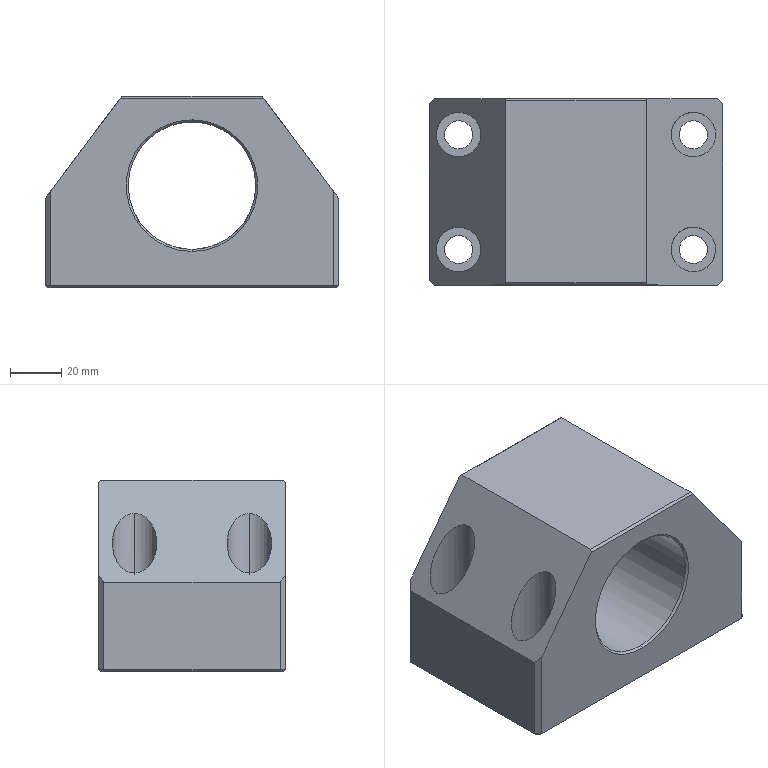Part | SolidWorks | features BaseBody 1 | 1 solid | 78 faces | box 115 x 73 x 75 mm | volume 354345 mm3 | plane 32 | cylinder 30 | cone 16 | commonest cylinder face diameters 6.5 x12 11 x8 17.5 x8 50 x2